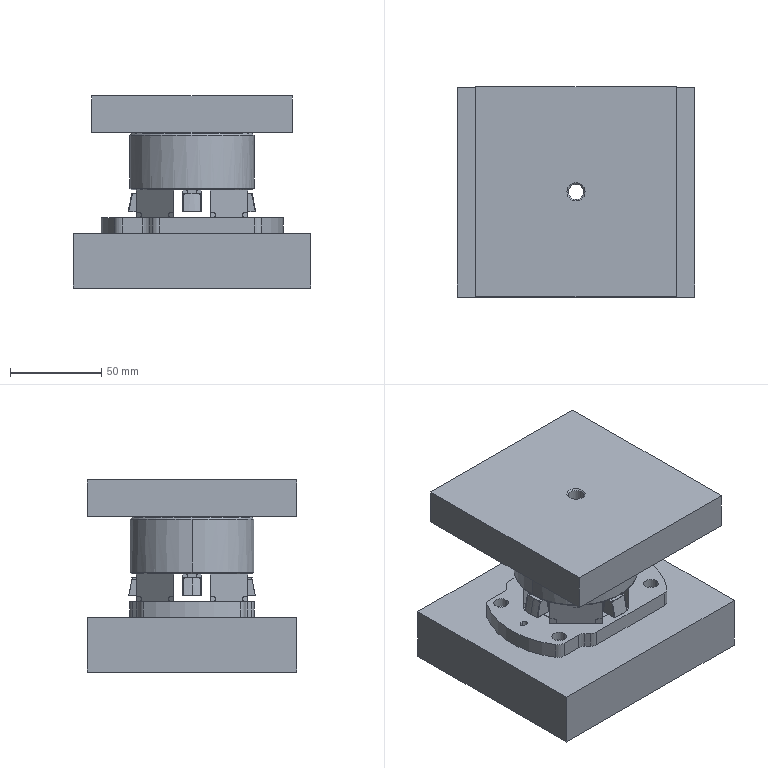NC program | NX | posted with a generic post | part box 130 x 115 x 105.2 mm
Lines 46 to 1308 of 3709:
(112 , TOOL : ER25-D4-32)
N78 T11 M6
N80 G54
N82 G17 G0 G90 X2.895 Y23.65 B0. C0. S5000 M3
N84 G43 Z105.2 H11
N86 G94 G1 Z54.7 F4500.
N88 G41 X2.9 Y27.55 F1500. D11
N90 Y27.625 F1375.
N92 Y27.7 F1250.
N94 Y27.775 F1125.
N96 Y27.85 F1000.
N98 Y27.925 F875.
N100 Y28. F750.
N102 X2.367
N104 X1.833 F1000.
N106 X1.3 F1250.
N108 X0.3 F1500.
N110 X-0.233 F1375.
N112 X-0.767 F1250.
N114 X-1.3 F1125.
N116 X-1.833 F1000.
N118 X-2.367 F875.
N120 X-2.9 F750.
N122 Y27.55
N124 Y23.95 F1500.
N126 G40
N128 X-2.895 Y23.65
N130 X2.895 Z54.2 F6000.
N132 G41 X2.9 Y27.55 F1500.
N134 Y27.625 F1375.
N136 Y27.7 F1250.
N138 Y27.775 F1125.
N140 Y27.85 F1000.
N142 Y27.925 F875.
N144 Y28. F750.
N146 X2.367
N148 X1.833 F1000.
N150 X1.3 F1250.
N152 X0.3 F1500.
N154 X-0.233 F1375.
N156 X-0.767 F1250.
N158 X-1.3 F1125.
N160 X-1.833 F1000.
N162 X-2.367 F875.
N164 X-2.9 F750.
N166 Y27.55
N168 Y23.95 F1500.
N170 G40
N172 X-2.895 Y23.65
N174 X2.895 Z53.7 F6000.
N176 G41 X2.9 Y27.55 F1500.
N178 Y27.625 F1375.
N180 Y27.7 F1250.
N182 Y27.775 F1125.
N184 Y27.85 F1000.
N186 Y27.925 F875.
N188 Y28. F750.
N190 X2.367
N192 X1.833 F1000.
N194 X1.3 F1250.
N196 X0.3 F1500.
N198 X-0.233 F1375.
N200 X-0.767 F1250.
N202 X-1.3 F1125.
N204 X-1.833 F1000.
N206 X-2.367 F875.
N208 X-2.9 F750.
N210 Y27.55
N212 Y23.95 F1500.
N214 G40
N216 X-2.895 Y23.65
N218 X2.895 Z53.2 F6000.
N220 G41 X2.9 Y27.55 F1500.
N222 Y27.625 F1375.
N224 Y27.7 F1250.
N226 Y27.775 F1125.
N228 Y27.85 F1000.
N230 Y27.925 F875.
N232 Y28. F750.
N234 X2.367
N236 X1.833 F1000.
N238 X1.3 F1250.
N240 X0.3 F1500.
N242 X-0.233 F1375.
N244 X-0.767 F1250.
N246 X-1.3 F1125.
N248 X-1.833 F1000.
N250 X-2.367 F875.
N252 X-2.9 F750.
N254 Y27.55
N256 Y23.95 F1500.
N258 G40
N260 X-2.895 Y23.65
N262 X2.895 Z52.7 F6000.
N264 G41 X2.9 Y27.55 F1500.
N266 Y27.625 F1375.
N268 Y27.7 F1250.
N270 Y27.775 F1125.
N272 Y27.85 F1000.
N274 Y27.925 F875.
N276 Y28. F750.
N278 X2.367
N280 X1.833 F1000.
N282 X1.3 F1250.
N284 X0.3 F1500.
N286 X-0.233 F1375.
N288 X-0.767 F1250.
N290 X-1.3 F1125.
N292 X-1.833 F1000.
N294 X-2.367 F875.
N296 X-2.9 F750.
N298 Y27.55
N300 Y23.95 F1500.
N302 G40
N304 X-2.895 Y23.65
N306 X2.895 Z52.2 F6000.
N308 G41 X2.9 Y27.55 F1500.
N310 Y27.625 F1375.
N312 Y27.7 F1250.
N314 Y27.775 F1125.
N316 Y27.85 F1000.
N318 Y27.925 F875.
N320 Y28. F750.
N322 X2.367
N324 X1.833 F1000.
N326 X1.3 F1250.
N328 X0.3 F1500.
N330 X-0.233 F1375.
N332 X-0.767 F1250.
N334 X-1.3 F1125.
N336 X-1.833 F1000.
N338 X-2.367 F875.
N340 X-2.9 F750.
N342 Y27.55
N344 Y23.95 F1500.
N346 G40
N348 X-2.895 Y23.65
N350 X2.895 Z51.7 F6000.
N352 G41 X2.9 Y27.55 F1500.
N354 Y27.625 F1375.
N356 Y27.7 F1250.
N358 Y27.775 F1125.
N360 Y27.85 F1000.
N362 Y27.925 F875.
N364 Y28. F750.
N366 X2.367
N368 X1.833 F1000.
N370 X1.3 F1250.
N372 X0.3 F1500.
N374 X-0.233 F1375.
N376 X-0.767 F1250.
N378 X-1.3 F1125.
N380 X-1.833 F1000.
N382 X-2.367 F875.
N384 X-2.9 F750.
N386 Y27.55
N388 Y23.95 F1500.
N390 G40
N392 X-2.895 Y23.65
N394 X2.895 Z51.2 F6000.
N396 G41 X2.9 Y27.55 F1500.
N398 Y27.625 F1375.
N400 Y27.7 F1250.
N402 Y27.775 F1125.
N404 Y27.85 F1000.
N406 Y27.925 F875.
N408 Y28. F750.
N410 X2.367
N412 X1.833 F1000.
N414 X1.3 F1250.
N416 X0.3 F1500.
N418 X-0.233 F1375.
N420 X-0.767 F1250.
N422 X-1.3 F1125.
N424 X-1.833 F1000.
N426 X-2.367 F875.
N428 X-2.9 F750.
N430 Y27.55
N432 Y23.95 F1500.
N434 G40
N436 X-2.895 Y23.65
N438 X2.895 Z50.7 F6000.
N440 G41 X2.9 Y27.55 F1500.
N442 Y27.625 F1375.
N444 Y27.7 F1250.
N446 Y27.775 F1125.
N448 Y27.85 F1000.
N450 Y27.925 F875.
N452 Y28. F750.
N454 X2.367
N456 X1.833 F1000.
N458 X1.3 F1250.
N460 X0.3 F1500.
N462 X-0.233 F1375.
N464 X-0.767 F1250.
N466 X-1.3 F1125.
N468 X-1.833 F1000.
N470 X-2.367 F875.
N472 X-2.9 F750.
N474 Y27.55
N476 Y23.95 F1500.
N478 G40
N480 X-2.895 Y23.65
N482 X2.895 Z50.2 F6000.
N484 G41 X2.9 Y27.55 F1500.
N486 Y27.625 F1375.
N488 Y27.7 F1250.
N490 Y27.775 F1125.
N492 Y27.85 F1000.
N494 Y27.925 F875.
N496 Y28. F750.
N498 X2.367
N500 X1.833 F1000.
N502 X1.3 F1250.
N504 X0.3 F1500.
N506 X-0.233 F1375.
N508 X-0.767 F1250.
N510 X-1.3 F1125.
N512 X-1.833 F1000.
N514 X-2.367 F875.
N516 X-2.9 F750.
N518 Y27.55
N520 Y23.95 F1500.
N522 G40
N524 X-2.895 Y23.65
N526 X2.895 Z49.7 F6000.
N528 G41 X2.9 Y27.55 F1500.
N530 Y27.625 F1375.
N532 Y27.7 F1250.
N534 Y27.775 F1125.
N536 Y27.85 F1000.
N538 Y27.925 F875.
N540 Y28. F750.
N542 X2.367
N544 X1.833 F1000.
N546 X1.3 F1250.
N548 X0.3 F1500.
N550 X-0.233 F1375.
N552 X-0.767 F1250.
N554 X-1.3 F1125.
N556 X-1.833 F1000.
N558 X-2.367 F875.
N560 X-2.9 F750.
N562 Y27.55
N564 Y23.95 F1500.
N566 G40
N568 X-2.895 Y23.65
N570 X2.895 Z49.2 F6000.
N572 G41 X2.9 Y27.55 F1500.
N574 Y27.625 F1375.
N576 Y27.7 F1250.
N578 Y27.775 F1125.
N580 Y27.85 F1000.
N582 Y27.925 F875.
N584 Y28. F750.
N586 X2.367
N588 X1.833 F1000.
N590 X1.3 F1250.
N592 X0.3 F1500.
N594 X-0.233 F1375.
N596 X-0.767 F1250.
N598 X-1.3 F1125.
N600 X-1.833 F1000.
N602 X-2.367 F875.
N604 X-2.9 F750.
N606 Y27.55
N608 Y23.95 F1500.
N610 G40
N612 X-2.895 Y23.65
N614 X2.895 Z48.7 F6000.
N616 G41 X2.9 Y27.55 F1500.
N618 Y27.625 F1375.
N620 Y27.7 F1250.
N622 Y27.775 F1125.
N624 Y27.85 F1000.
N626 Y27.925 F875.
N628 Y28. F750.
N630 X2.367
N632 X1.833 F1000.
N634 X1.3 F1250.
N636 X0.3 F1500.
N638 X-0.233 F1375.
N640 X-0.767 F1250.
N642 X-1.3 F1125.
N644 X-1.833 F1000.
N646 X-2.367 F875.
N648 X-2.9 F750.
N650 Y27.55
N652 Y23.95 F1500.
N654 G40
N656 X-2.895 Y23.65
N658 X2.895 Z48.2 F6000.
N660 G41 X2.9 Y27.55 F1500.
N662 Y27.625 F1375.
N664 Y27.7 F1250.
N666 Y27.775 F1125.
N668 Y27.85 F1000.
N670 Y27.925 F875.
N672 Y28. F750.
N674 X2.367
N676 X1.833 F1000.
N678 X1.3 F1250.
N680 X0.3 F1500.
N682 X-0.233 F1375.
N684 X-0.767 F1250.
N686 X-1.3 F1125.
N688 X-1.833 F1000.
N690 X-2.367 F875.
N692 X-2.9 F750.
N694 Y27.55
N696 Y23.95 F1500.
N698 G40
N700 X-2.895 Y23.65
N702 X2.895 Z47.7 F6000.
N704 G41 X2.9 Y27.55 F1500.
N706 Y27.625 F1375.
N708 Y27.7 F1250.
N710 Y27.775 F1125.
N712 Y27.85 F1000.
N714 Y27.925 F875.
N716 Y28. F750.
N718 X2.367
N720 X1.833 F1000.
N722 X1.3 F1250.
N724 X0.3 F1500.
N726 X-0.233 F1375.
N728 X-0.767 F1250.
N730 X-1.3 F1125.
N732 X-1.833 F1000.
N734 X-2.367 F875.
N736 X-2.9 F750.
N738 Y27.55
N740 Y23.95 F1500.
N742 G40
N744 X-2.895 Y23.65
N746 X2.895 Z47.2 F6000.
N748 G41 X2.9 Y27.55 F1500.
N750 Y27.625 F1375.
N752 Y27.7 F1250.
N754 Y27.775 F1125.
N756 Y27.85 F1000.
N758 Y27.925 F875.
N760 Y28. F750.
N762 X2.367
N764 X1.833 F1000.
N766 X1.3 F1250.
N768 X0.3 F1500.
N770 X-0.233 F1375.
N772 X-0.767 F1250.
N774 X-1.3 F1125.
N776 X-1.833 F1000.
N778 X-2.367 F875.
N780 X-2.9 F750.
N782 Y27.55
N784 Y23.95 F1500.
N786 G40
N788 X-2.895 Y23.65
N790 X2.895 Z46.7 F6000.
N792 G41 X2.9 Y27.55 F1500.
N794 Y27.625 F1375.
N796 Y27.7 F1250.
N798 Y27.775 F1125.
N800 Y27.85 F1000.
N802 Y27.925 F875.
N804 Y28. F750.
N806 X2.367
N808 X1.833 F1000.
N810 X1.3 F1250.
N812 X0.3 F1500.
N814 X-0.233 F1375.
N816 X-0.767 F1250.
N818 X-1.3 F1125.
N820 X-1.833 F1000.
N822 X-2.367 F875.
N824 X-2.9 F750.
N826 Y27.55
N828 Y23.95 F1500.
N830 G40
N832 X-2.895 Y23.65
N834 X2.895 Z46.2 F6000.
N836 G41 X2.9 Y27.55 F1500.
N838 Y27.625 F1375.
N840 Y27.7 F1250.
N842 Y27.775 F1125.
N844 Y27.85 F1000.
N846 Y27.925 F875.
N848 Y28. F750.
N850 X2.367
N852 X1.833 F1000.
N854 X1.3 F1250.
N856 X0.3 F1500.
N858 X-0.233 F1375.
N860 X-0.767 F1250.
N862 X-1.3 F1125.
N864 X-1.833 F1000.
N866 X-2.367 F875.
N868 X-2.9 F750.
N870 Y27.55
N872 Y23.95 F1500.
N874 G40
N876 X-2.895 Y23.65
N878 X2.895 Z45.7 F6000.
N880 G41 X2.9 Y27.55 F1500.
N882 Y27.625 F1375.
N884 Y27.7 F1250.
N886 Y27.775 F1125.
N888 Y27.85 F1000.
N890 Y27.925 F875.
N892 Y28. F750.
N894 X2.367
N896 X1.833 F1000.
N898 X1.3 F1250.
N900 X0.3 F1500.
N902 X-0.233 F1375.
N904 X-0.767 F1250.
N906 X-1.3 F1125.
N908 X-1.833 F1000.
N910 X-2.367 F875.
N912 X-2.9 F750.
N914 Y27.55
N916 Y23.95 F1500.
N918 G40
N920 X-2.895 Y23.65
N922 X2.895 Z45.2 F6000.
N924 G41 X2.9 Y27.55 F1500.
N926 Y27.625 F1375.
N928 Y27.7 F1250.
N930 Y27.775 F1125.
N932 Y27.85 F1000.
N934 Y27.925 F875.
N936 Y28. F750.
N938 X2.367
N940 X1.833 F1000.
N942 X1.3 F1250.
N944 X0.3 F1500.
N946 X-0.233 F1375.
N948 X-0.767 F1250.
N950 X-1.3 F1125.
N952 X-1.833 F1000.
N954 X-2.367 F875.
N956 X-2.9 F750.
N958 Y27.55
N960 Y23.95 F1500.
N962 G40
N964 X-2.895 Y23.65
N966 X2.895 Z44.7 F6000.
N968 G41 X2.9 Y27.55 F1500.
N970 Y27.625 F1375.
N972 Y27.7 F1250.
N974 Y27.775 F1125.
N976 Y27.85 F1000.
N978 Y27.925 F875.
N980 Y28. F750.
N982 X2.367
N984 X1.833 F1000.
N986 X1.3 F1250.
N988 X0.3 F1500.
N990 X-0.233 F1375.
N992 X-0.767 F1250.
N994 X-1.3 F1125.
N996 X-1.833 F1000.
N998 X-2.367 F875.
N1000 X-2.9 F750.
N1002 Y27.55
N1004 Y23.95 F1500.
N1006 G40
N1008 X-2.895 Y23.65
N1010 X2.895 Z44.2 F6000.
N1012 G41 X2.9 Y27.55 F1500.
N1014 Y27.625 F1375.
N1016 Y27.7 F1250.
N1018 Y27.775 F1125.
N1020 Y27.85 F1000.
N1022 Y27.925 F875.
N1024 Y28. F750.
N1026 X2.367
N1028 X1.833 F1000.
N1030 X1.3 F1250.
N1032 X0.3 F1500.
N1034 X-0.233 F1375.
N1036 X-0.767 F1250.
N1038 X-1.3 F1125.
N1040 X-1.833 F1000.
N1042 X-2.367 F875.
N1044 X-2.9 F750.
N1046 Y27.55
N1048 Y23.95 F1500.
N1050 G40
N1052 X-2.895 Y23.65
N1054 X2.895 Z43.7 F6000.
N1056 G41 X2.9 Y27.55 F1500.
N1058 Y27.625 F1375.
N1060 Y27.7 F1250.
N1062 Y27.775 F1125.
N1064 Y27.85 F1000.
N1066 Y27.925 F875.
N1068 Y28. F750.
N1070 X2.367
N1072 X1.833 F1000.
N1074 X1.3 F1250.
N1076 X0.3 F1500.
N1078 X-0.233 F1375.
N1080 X-0.767 F1250.
N1082 X-1.3 F1125.
N1084 X-1.833 F1000.
N1086 X-2.367 F875.
N1088 X-2.9 F750.
N1090 Y27.55
N1092 Y23.95 F1500.
N1094 G40
N1096 X-2.895 Y23.65
N1098 X2.895 Z43.2 F6000.
N1100 G41 X2.9 Y27.55 F1500.
N1102 Y27.625 F1375.
N1104 Y27.7 F1250.
N1106 Y27.775 F1125.
N1108 Y27.85 F1000.
N1110 Y27.925 F875.
N1112 Y28. F750.
N1114 X2.367
N1116 X1.833 F1000.
N1118 X1.3 F1250.
N1120 X0.3 F1500.
N1122 X-0.233 F1375.
N1124 X-0.767 F1250.
N1126 X-1.3 F1125.
N1128 X-1.833 F1000.
N1130 X-2.367 F875.
N1132 X-2.9 F750.
N1134 Y27.55
N1136 Y23.95 F1500.
N1138 G40
N1140 X-2.895 Y23.65
N1142 X2.895 Z42.7 F6000.
N1144 G41 X2.9 Y27.55 F1500.
N1146 Y27.625 F1375.
N1148 Y27.7 F1250.
N1150 Y27.775 F1125.
N1152 Y27.85 F1000.
N1154 Y27.925 F875.
N1156 Y28. F750.
N1158 X2.367
N1160 X1.833 F1000.
N1162 X1.3 F1250.
N1164 X0.3 F1500.
N1166 X-0.233 F1375.
N1168 X-0.767 F1250.
N1170 X-1.3 F1125.
N1172 X-1.833 F1000.
N1174 X-2.367 F875.
N1176 X-2.9 F750.
N1178 Y27.55
N1180 Y23.95 F1500.
N1182 G40
N1184 X-2.895 Y23.65
N1186 X2.895 Z42.2 F6000.
N1188 G41 X2.9 Y27.55 F1500.
N1190 Y27.625 F1375.
N1192 Y27.7 F1250.
N1194 Y27.775 F1125.
N1196 Y27.85 F1000.
N1198 Y27.925 F875.
N1200 Y28. F750.
N1202 X2.367
N1204 X1.833 F1000.
N1206 X1.3 F1250.
N1208 X0.3 F1500.
N1210 X-0.233 F1375.
N1212 X-0.767 F1250.
N1214 X-1.3 F1125.
N1216 X-1.833 F1000.
N1218 X-2.367 F875.
N1220 X-2.9 F750.
N1222 Y27.55
N1224 Y23.95 F1500.
N1226 G40
N1228 X-2.895 Y23.65
N1230 X2.895 Z41.7 F6000.
N1232 G41 X2.9 Y27.55 F1500.
N1234 Y27.625 F1375.
N1236 Y27.7 F1250.
N1238 Y27.775 F1125.
N1240 Y27.85 F1000.
N1242 Y27.925 F875.
N1244 Y28. F750.
N1246 X2.367
N1248 X1.833 F1000.
N1250 X1.3 F1250.
N1252 X0.3 F1500.
N1254 X-0.233 F1375.
N1256 X-0.767 F1250.
N1258 X-1.3 F1125.
N1260 X-1.833 F1000.
N1262 X-2.367 F875.
N1264 X-2.9 F750.
N1266 Y27.55
N1268 Y23.95 F1500.
N1270 G40
N1272 X-2.895 Y23.65
N1274 X2.895 Z41.2 F6000.
N1276 G41 X2.9 Y27.55 F1500.
N1278 Y27.625 F1375.
N1280 Y27.7 F1250.
N1282 Y27.775 F1125.
N1284 Y27.85 F1000.
N1286 Y27.925 F875.
N1288 Y28. F750.
N1290 X2.367
N1292 X1.833 F1000.
N1294 X1.3 F1250.
N1296 X0.3 F1500.
N1298 X-0.233 F1375.
N1300 X-0.767 F1250.
N1302 X-1.3 F1125.
N1304 X-1.833 F1000.
N1306 X-2.367 F875.
N1308 X-2.9 F750.
N1310 Y27.55
N1312 Y23.95 F1500.
N1314 G40
N1316 X-2.895 Y23.65
N1318 X2.895 Z40.7 F6000.
N1320 G41 X2.9 Y27.55 F1500.
N1322 Y27.625 F1375.
N1324 Y27.7 F1250.
N1326 Y27.775 F1125.
N1328 Y27.85 F1000.
N1330 Y27.925 F875.
N1332 Y28. F750.
N1334 X2.367
N1336 X1.833 F1000.
N1338 X1.3 F1250.
N1340 X0.3 F1500.
N1342 X-0.233 F1375.
N1344 X-0.767 F1250.
N1346 X-1.3 F1125.
N1348 X-1.833 F1000.
N1350 X-2.367 F875.
N1352 X-2.9 F750.
N1354 Y27.55
N1356 Y23.95 F1500.
N1358 G40
N1360 X-2.895 Y23.65
N1362 X2.895 Z40.2 F6000.
N1364 G41 X2.9 Y27.55 F1500.
N1366 Y27.625 F1375.
N1368 Y27.7 F1250.
N1370 Y27.775 F1125.
N1372 Y27.85 F1000.
N1374 Y27.925 F875.
N1376 Y28. F750.
N1378 X2.367
N1380 X1.833 F1000.
N1382 X1.3 F1250.
N1384 X0.3 F1500.
N1386 X-0.233 F1375.
N1388 X-0.767 F1250.
N1390 X-1.3 F1125.
N1392 X-1.833 F1000.
N1394 X-2.367 F875.
N1396 X-2.9 F750.
N1398 Y27.55
N1400 Y23.95 F1500.
N1402 G40
N1404 X-2.895 Y23.65
N1406 X2.895 Z39.7 F6000.
N1408 G41 X2.9 Y27.55 F1500.
N1410 Y27.625 F1375.
N1412 Y27.7 F1250.
N1414 Y27.775 F1125.
N1416 Y27.85 F1000.
N1418 Y27.925 F875.
N1420 Y28. F750.
N1422 X2.367
N1424 X1.833 F1000.
N1426 X1.3 F1250.
N1428 X0.3 F1500.
N1430 X-0.233 F1375.
N1432 X-0.767 F1250.
N1434 X-1.3 F1125.
N1436 X-1.833 F1000.
N1438 X-2.367 F875.
N1440 X-2.9 F750.
N1442 Y27.55
N1444 Y23.95 F1500.
N1446 G40
N1448 X-2.895 Y23.65
N1450 X2.895 Z39.2 F6000.
N1452 G41 X2.9 Y27.55 F1500.
N1454 Y27.625 F1375.
N1456 Y27.7 F1250.
N1458 Y27.775 F1125.
N1460 Y27.85 F1000.
N1462 Y27.925 F875.
N1464 Y28. F750.
N1466 X2.367
N1468 X1.833 F1000.
N1470 X1.3 F1250.
N1472 X0.3 F1500.
N1474 X-0.233 F1375.
N1476 X-0.767 F1250.
N1478 X-1.3 F1125.
N1480 X-1.833 F1000.
N1482 X-2.367 F875.
N1484 X-2.9 F750.
N1486 Y27.55
N1488 Y23.95 F1500.
N1490 G40
N1492 X-2.895 Y23.65
N1494 X2.895 Z38.7 F6000.
N1496 G41 X2.9 Y27.55 F1500.
N1498 Y27.625 F1375.
N1500 Y27.7 F1250.
N1502 Y27.775 F1125.
N1504 Y27.85 F1000.
N1506 Y27.925 F875.
N1508 Y28. F750.
N1510 X2.367
N1512 X1.833 F1000.
N1514 X1.3 F1250.
N1516 X0.3 F1500.
N1518 X-0.233 F1375.
N1520 X-0.767 F1250.
N1522 X-1.3 F1125.
N1524 X-1.833 F1000.
N1526 X-2.367 F875.
N1528 X-2.9 F750.
N1530 Y27.55
N1532 Y23.95 F1500.
N1534 G40
N1536 X-2.895 Y23.65
N1538 X2.895 Z38.2 F6000.
N1540 G41 X2.9 Y27.55 F1500.
N1542 Y27.625 F1375.
N1544 Y27.7 F1250.
N1546 Y27.775 F1125.
N1548 Y27.85 F1000.
N1550 Y27.925 F875.
N1552 Y28. F750.
N1554 X2.367
N1556 X1.833 F1000.
N1558 X1.3 F1250.
N1560 X0.3 F1500.
N1562 X-0.233 F1375.
N1564 X-0.767 F1250.
N1566 X-1.3 F1125.
N1568 X-1.833 F1000.
N1570 X-2.367 F875.
N1572 X-2.9 F750.
N1574 Y27.55
N1576 Y23.95 F1500.
N1578 G40
N1580 X-2.895 Y23.65
N1582 X2.895 Z37.7 F6000.
N1584 G41 X2.9 Y27.55 F1500.
N1586 Y27.625 F1375.
N1588 Y27.7 F1250.
N1590 Y27.775 F1125.
N1592 Y27.85 F1000.
N1594 Y27.925 F875.
N1596 Y28. F750.
N1598 X2.367
N1600 X1.833 F1000.
N1602 X1.3 F1250.
N1604 X0.3 F1500.
N1606 X-0.233 F1375.
N1608 X-0.767 F1250.
N1610 X-1.3 F1125.
N1612 X-1.833 F1000.
N1614 X-2.367 F875.
N1616 X-2.9 F750.
N1618 Y27.55
N1620 Y23.95 F1500.
N1622 G40
N1624 X-2.895 Y23.65
N1626 X2.895 Z37.2 F6000.
N1628 G41 X2.9 Y27.55 F1500.
N1630 Y27.625 F1375.
N1632 Y27.7 F1250.
N1634 Y27.775 F1125.
N1636 Y27.85 F1000.
N1638 Y27.925 F875.
N1640 Y28. F750.
N1642 X2.367
N1644 X1.833 F1000.
N1646 X1.3 F1250.
N1648 X0.3 F1500.
N1650 X-0.233 F1375.
N1652 X-0.767 F1250.
N1654 X-1.3 F1125.
N1656 X-1.833 F1000.
N1658 X-2.367 F875.
N1660 X-2.9 F750.
N1662 Y27.55
N1664 Y23.95 F1500.
N1666 G40
N1668 X-2.895 Y23.65
N1670 X2.895 Z36.7 F6000.
N1672 G41 X2.9 Y27.55 F1500.
N1674 Y27.625 F1375.
N1676 Y27.7 F1250.
N1678 Y27.775 F1125.
N1680 Y27.85 F1000.
N1682 Y27.925 F875.
N1684 Y28. F750.
N1686 X2.367
N1688 X1.833 F1000.
N1690 X1.3 F1250.
N1692 X0.3 F1500.
N1694 X-0.233 F1375.
N1696 X-0.767 F1250.
N1698 X-1.3 F1125.
N1700 X-1.833 F1000.
N1702 X-2.367 F875.
N1704 X-2.9 F750.
N1706 Y27.55
N1708 Y23.95 F1500.
N1710 G40
N1712 X-2.895 Y23.65
N1714 X2.895 Z36.2 F6000.
N1716 G41 X2.9 Y27.55 F1500.
N1718 Y27.625 F1375.
N1720 Y27.7 F1250.
N1722 Y27.775 F1125.
N1724 Y27.85 F1000.
N1726 Y27.925 F875.
N1728 Y28. F750.
N1730 X2.367
N1732 X1.833 F1000.
N1734 X1.3 F1250.
N1736 X0.3 F1500.
N1738 X-0.233 F1375.
N1740 X-0.767 F1250.
N1742 X-1.3 F1125.
N1744 X-1.833 F1000.
N1746 X-2.367 F875.
N1748 X-2.9 F750.
N1750 Y27.55
N1752 Y23.95 F1500.
N1754 G40
N1756 X-2.895 Y23.65
N1758 X2.895 Z35.7 F6000.
N1760 G41 X2.9 Y27.55 F1500.
N1762 Y27.625 F1375.
N1764 Y27.7 F1250.
N1766 Y27.775 F1125.
N1768 Y27.85 F1000.
N1770 Y27.925 F875.
N1772 Y28. F750.
N1774 X2.367
N1776 X1.833 F1000.
N1778 X1.3 F1250.
N1780 X0.3 F1500.
N1782 X-0.233 F1375.
N1784 X-0.767 F1250.
N1786 X-1.3 F1125.
N1788 X-1.833 F1000.
N1790 X-2.367 F875.
N1792 X-2.9 F750.
N1794 Y27.55
N1796 Y23.95 F1500.
N1798 G40
N1800 X-2.895 Y23.65
N1802 X2.895 Z35.2 F6000.
N1804 G41 X2.9 Y27.55 F1500.
N1806 Y27.625 F1375.
N1808 Y27.7 F1250.
N1810 Y27.775 F1125.
N1812 Y27.85 F1000.
N1814 Y27.925 F875.
N1816 Y28. F750.
N1818 X2.367
N1820 X1.833 F1000.
N1822 X1.3 F1250.
N1824 X0.3 F1500.
N1826 X-0.233 F1375.
N1828 X-0.767 F1250.
N1830 X-1.3 F1125.
N1832 X-1.833 F1000.
N1834 X-2.367 F875.
N1836 X-2.9 F750.
N1838 Y27.55
N1840 Y23.95 F1500.
N1842 G40
N1844 X-2.895 Y23.65
N1846 X2.895 Z34.7 F6000.
N1848 G41 X2.9 Y27.55 F1500.
N1850 Y27.625 F1375.
N1852 Y27.7 F1250.
N1854 Y27.775 F1125.
N1856 Y27.85 F1000.
N1858 Y27.925 F875.
N1860 Y28. F750.
N1862 X2.367
N1864 X1.833 F1000.
N1866 X1.3 F1250.
N1868 X0.3 F1500.
N1870 X-0.233 F1375.
N1872 X-0.767 F1250.
N1874 X-1.3 F1125.
N1876 X-1.833 F1000.
N1878 X-2.367 F875.
N1880 X-2.9 F750.
N1882 Y27.55
N1884 Y23.95 F1500.
N1886 G40
N1888 X-2.895 Y23.65
N1890 X2.895 Z34.2 F6000.
N1892 G41 X2.9 Y27.55 F1500.
N1894 Y27.625 F1375.
N1896 Y27.7 F1250.
N1898 Y27.775 F1125.
N1900 Y27.85 F1000.
N1902 Y27.925 F875.
N1904 Y28. F750.
N1906 X2.367
N1908 X1.833 F1000.
N1910 X1.3 F1250.
N1912 X0.3 F1500.
N1914 X-0.233 F1375.
N1916 X-0.767 F1250.
N1918 X-1.3 F1125.
N1920 X-1.833 F1000.
N1922 X-2.367 F875.
N1924 X-2.9 F750.
N1926 Y27.55
N1928 Y23.95 F1500.
N1930 G40
N1932 X-2.895 Y23.65
N1934 X2.895 Z33.7 F6000.
N1936 G41 X2.9 Y27.55 F1500.
N1938 Y27.625 F1375.
N1940 Y27.7 F1250.
N1942 Y27.775 F1125.
N1944 Y27.85 F1000.
N1946 Y27.925 F875.
N1948 Y28. F750.
N1950 X2.367
N1952 X1.833 F1000.
N1954 X1.3 F1250.
N1956 X0.3 F1500.
N1958 X-0.233 F1375.
N1960 X-0.767 F1250.
N1962 X-1.3 F1125.
N1964 X-1.833 F1000.
N1966 X-2.367 F875.
N1968 X-2.9 F750.
N1970 Y27.55
N1972 Y23.95 F1500.
N1974 G40
N1976 X-2.895 Y23.65
N1978 X2.895 Z33.2 F6000.
N1980 G41 X2.9 Y27.55 F1500.
N1982 Y27.625 F1375.
N1984 Y27.7 F1250.
N1986 Y27.775 F1125.
N1988 Y27.85 F1000.
N1990 Y27.925 F875.
N1992 Y28. F750.
N1994 X2.367
N1996 X1.833 F1000.
N1998 X1.3 F1250.
N2000 X0.3 F1500.
N2002 X-0.233 F1375.
N2004 X-0.767 F1250.
N2006 X-1.3 F1125.
N2008 X-1.833 F1000.
N2010 X-2.367 F875.
N2012 X-2.9 F750.
N2014 Y27.55
N2016 Y23.95 F1500.
N2018 G40
N2020 X-2.895 Y23.65
N2022 X2.895 Z32.7 F6000.
N2024 G41 X2.9 Y27.55 F1500.
N2026 Y27.625 F1375.
N2028 Y27.7 F1250.
N2030 Y27.775 F1125.
N2032 Y27.85 F1000.
N2034 Y27.925 F875.
N2036 Y28. F750.
N2038 X2.367
N2040 X1.833 F1000.
N2042 X1.3 F1250.
N2044 X0.3 F1500.
N2046 X-0.233 F1375.
N2048 X-0.767 F1250.
N2050 X-1.3 F1125.
N2052 X-1.833 F1000.
N2054 X-2.367 F875.
N2056 X-2.9 F750.
N2058 Y27.55
N2060 Y23.95 F1500.
N2062 G40
N2064 X-2.895 Y23.65
N2066 X2.895 Z32.2 F6000.
N2068 G41 X2.9 Y27.55 F1500.
N2070 Y27.625 F1375.
N2072 Y27.7 F1250.
N2074 Y27.775 F1125.
N2076 Y27.85 F1000.
N2078 Y27.925 F875.
N2080 Y28. F750.
N2082 X2.367
N2084 X1.833 F1000.
N2086 X1.3 F1250.
N2088 X0.3 F1500.
N2090 X-0.233 F1375.
N2092 X-0.767 F1250.
N2094 X-1.3 F1125.
N2096 X-1.833 F1000.
N2098 X-2.367 F875.
N2100 X-2.9 F750.
N2102 Y27.55
N2104 Y23.95 F1500.
N2106 G40
N2108 X-2.895 Y23.65
N2110 X2.895 Z31.7 F6000.
N2112 G41 X2.9 Y27.55 F1500.
N2114 Y27.625 F1375.
N2116 Y27.7 F1250.
N2118 Y27.775 F1125.
N2120 Y27.85 F1000.
N2122 Y27.925 F875.
N2124 Y28. F750.
N2126 X2.367
N2128 X1.833 F1000.
N2130 X1.3 F1250.
N2132 X0.3 F1500.
N2134 X-0.233 F1375.
N2136 X-0.767 F1250.
N2138 X-1.3 F1125.
N2140 X-1.833 F1000.
N2142 X-2.367 F875.
N2144 X-2.9 F750.
N2146 Y27.55
N2148 Y23.95 F1500.
N2150 G40
N2152 X-2.895 Y23.65
N2154 X2.895 Z31.2 F6000.
N2156 G41 X2.9 Y27.55 F1500.
N2158 Y27.625 F1375.
N2160 Y27.7 F1250.
N2162 Y27.775 F1125.
N2164 Y27.85 F1000.
N2166 Y27.925 F875.
N2168 Y28. F750.
N2170 X2.367
N2172 X1.833 F1000.
N2174 X1.3 F1250.
N2176 X0.3 F1500.
N2178 X-0.233 F1375.
N2180 X-0.767 F1250.
N2182 X-1.3 F1125.
N2184 X-1.833 F1000.
N2186 X-2.367 F875.
N2188 X-2.9 F750.
N2190 Y27.55
N2192 Y23.95 F1500.
N2194 G40
N2196 X-2.895 Y23.65
N2198 X2.895 Z30.7 F6000.
N2200 G41 X2.9 Y27.55 F1500.
N2202 Y27.625 F1375.
N2204 Y27.7 F1250.
N2206 Y27.775 F1125.
N2208 Y27.85 F1000.
N2210 Y27.925 F875.
N2212 Y28. F750.
N2214 X2.367
N2216 X1.833 F1000.
N2218 X1.3 F1250.
N2220 X0.3 F1500.
N2222 X-0.233 F1375.
N2224 X-0.767 F1250.
N2226 X-1.3 F1125.
N2228 X-1.833 F1000.
N2230 X-2.367 F875.
N2232 X-2.9 F750.
N2234 Y27.55
N2236 Y23.95 F1500.
N2238 G40
N2240 X-2.895 Y23.65
N2242 X2.895 Z30.2 F6000.
N2244 G41 X2.9 Y27.55 F1500.
N2246 Y27.625 F1375.
N2248 Y27.7 F1250.
N2250 Y27.775 F1125.
N2252 Y27.85 F1000.
N2254 Y27.925 F875.
N2256 Y28. F750.
N2258 X2.367
N2260 X1.833 F1000.
N2262 X1.3 F1250.
N2264 X0.3 F1500.
N2266 X-0.233 F1375.
N2268 X-0.767 F1250.
N2270 X-1.3 F1125.
N2272 X-1.833 F1000.
N2274 X-2.367 F875.
N2276 X-2.9 F750.
N2278 Y27.55
N2280 Y23.95 F1500.
N2282 G40
N2284 X-2.895 Y23.65
N2286 X2.895 Z29.7 F6000.
N2288 G41 X2.9 Y27.55 F1500.
N2290 Y27.625 F1375.
N2292 Y27.7 F1250.
N2294 Y27.775 F1125.
N2296 Y27.85 F1000.
N2298 Y27.925 F875.
N2300 Y28. F750.
N2302 X2.367
N2304 X1.833 F1000.
N2306 X1.3 F1250.
N2308 X0.3 F1500.
N2310 X-0.233 F1375.
N2312 X-0.767 F1250.
N2314 X-1.3 F1125.
N2316 X-1.833 F1000.
N2318 X-2.367 F875.
N2320 X-2.9 F750.
N2322 Y27.55
N2324 Y23.95 F1500.
N2326 G40
N2328 X-2.895 Y23.65
N2330 X2.895 Z29.2 F6000.
N2332 G41 X2.9 Y27.55 F1500.
N2334 Y27.625 F1375.
N2336 Y27.7 F1250.
N2338 Y27.775 F1125.
N2340 Y27.85 F1000.
N2342 Y27.925 F875.
N2344 Y28. F750.
N2346 X2.367
N2348 X1.833 F1000.
N2350 X1.3 F1250.
N2352 X0.3 F1500.
N2354 X-0.233 F1375.
N2356 X-0.767 F1250.
N2358 X-1.3 F1125.
N2360 X-1.833 F1000.
N2362 X-2.367 F875.
N2364 X-2.9 F750.
N2366 Y27.55
N2368 Y23.95 F1500.
N2370 G40
N2372 X-2.895 Y23.65
N2374 X2.895 Z28.7 F6000.
N2376 G41 X2.9 Y27.55 F1500.
N2378 Y27.625 F1375.
N2380 Y27.7 F1250.
N2382 Y27.775 F1125.
N2384 Y27.85 F1000.
N2386 Y27.925 F875.
N2388 Y28. F750.
N2390 X2.367
N2392 X1.833 F1000.
N2394 X1.3 F1250.
N2396 X0.3 F1500.
N2398 X-0.233 F1375.
N2400 X-0.767 F1250.
N2402 X-1.3 F1125.
N2404 X-1.833 F1000.
N2406 X-2.367 F875.
N2408 X-2.9 F750.
N2410 Y27.55
N2412 Y23.95 F1500.
N2414 G40
N2416 X-2.895 Y23.65
N2418 X2.895 Z28.2 F6000.
N2420 G41 X2.9 Y27.55 F1500.
N2422 Y27.625 F1375.
N2424 Y27.7 F1250.
N2426 Y27.775 F1125.
N2428 Y27.85 F1000.
N2430 Y27.925 F875.
N2432 Y28. F750.
N2434 X2.367
N2436 X1.833 F1000.
N2438 X1.3 F1250.
N2440 X0.3 F1500.
N2442 X-0.233 F1375.
N2444 X-0.767 F1250.
N2446 X-1.3 F1125.
N2448 X-1.833 F1000.
N2450 X-2.367 F875.
N2452 X-2.9 F750.
N2454 Y27.55
N2456 Y23.95 F1500.
N2458 G40
N2460 X-2.895 Y23.65
N2462 X2.895 Z27.7 F6000.
N2464 G41 X2.9 Y27.55 F1500.
N2466 Y27.625 F1375.
N2468 Y27.7 F1250.
N2470 Y27.775 F1125.
N2472 Y27.85 F1000.
N2474 Y27.925 F875.
N2476 Y28. F750.
N2478 X2.367
N2480 X1.833 F1000.
N2482 X1.3 F1250.
N2484 X0.3 F1500.
N2486 X-0.233 F1375.
N2488 X-0.767 F1250.
N2490 X-1.3 F1125.
N2492 X-1.833 F1000.
N2494 X-2.367 F875.
N2496 X-2.9 F750.
N2498 Y27.55
N2500 Y23.95 F1500.
N2502 G40
N2504 X-2.895 Y23.65
N2506 X2.895 Z27.2 F6000.
N2508 G41 X2.9 Y27.55 F1500.
N2510 Y27.625 F1375.
N2512 Y27.7 F1250.
N2514 Y27.775 F1125.
N2516 Y27.85 F1000.
N2518 Y27.925 F875.
N2520 Y28. F750.
N2522 X2.367
N2524 X1.833 F1000.
N2526 X1.3 F1250.
N2528 X0.3 F1500.
N2530 X-0.233 F1375.
N2532 X-0.767 F1250.
N2534 X-1.3 F1125.
N2536 X-1.833 F1000.
N2538 X-2.367 F875.
N2540 X-2.9 F750.
N2542 Y27.55
N2544 Y23.95 F1500.
N2546 G40
N2548 X-2.895 Y23.65
N2550 X2.895 Z26.7 F6000.
N2552 G41 X2.9 Y27.55 F1500.
N2554 Y27.625 F1375.
N2556 Y27.7 F1250.
N2558 Y27.775 F1125.
N2560 Y27.85 F1000.
N2562 Y27.925 F875.
N2564 Y28. F750.
N2566 X2.367
N2568 X1.833 F1000.
N2570 X1.3 F1250.
N2572 X0.3 F1500.
N2574 X-0.233 F1375.
N2576 X-0.767 F1250.
N2578 X-1.3 F1125.
N2580 X-1.833 F1000.
N2582 X-2.367 F875.
N2584 X-2.9 F750.
N2586 Y27.55
N2588 Y23.95 F1500.
N2590 G40
N2592 X-2.895 Y23.65
N2594 X2.895 Z26.2 F6000.
N2596 G41 X2.9 Y27.55 F1500.